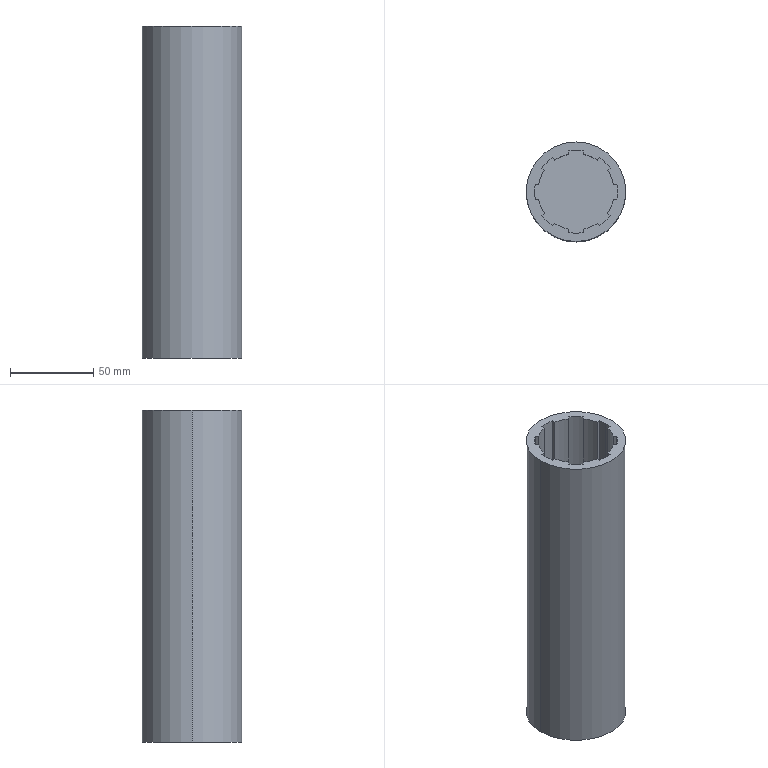Part | SolidWorks | features ICE 2, Extrusion 1 | 1 solid | 72 faces | box 60 x 60 x 200 mm | volume 299813 mm3 | cylinder 36 | plane 36 | commonest cylinder face diameters 46 x17 50 x9 42 x8 60 x2